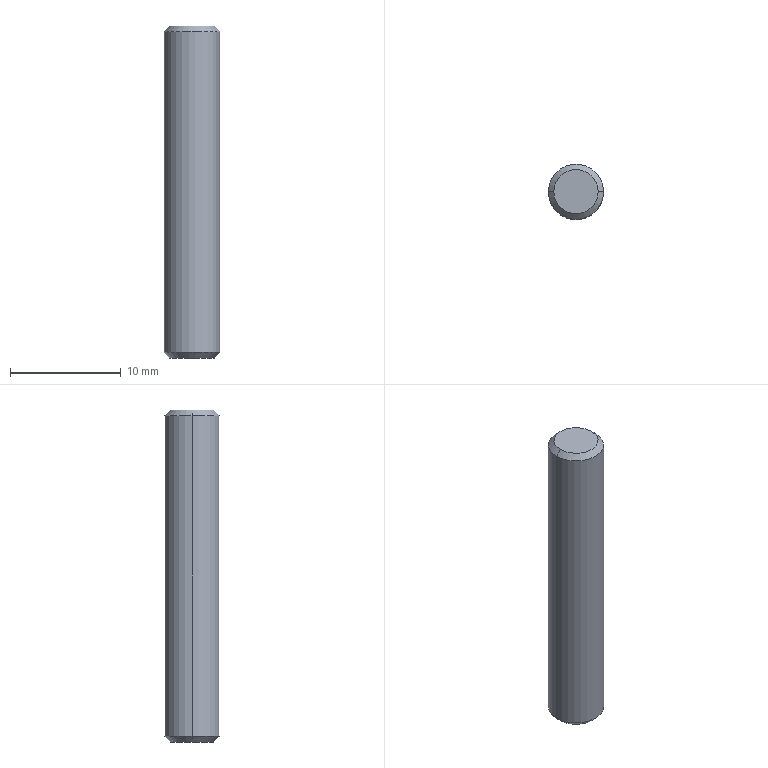Part | SolidWorks | features Chamfer 1, Extrusion 1 | 1 solid | 8 faces | box 5 x 5 x 30 mm | volume 585.383 mm3 | cone 4 | cylinder 2 | plane 2 | commonest cylinder face diameters 5 x2
STEP:
#1=CARTESIAN_POINT('',(-2.,0.,-15.));
#2=VERTEX_POINT('',#1);
#3=CARTESIAN_POINT('',(2.,0.,-15.));
#4=VERTEX_POINT('',#3);
#5=CARTESIAN_POINT('',(0.,0.,-15.));
#6=DIRECTION('',(0.,0.,-1.));
#7=DIRECTION('',(1.,0.,0.));
#8=AXIS2_PLACEMENT_3D('',#5,#6,#7);
#9=CIRCLE('',#8,2.);
#10=EDGE_CURVE('',#2,#4,#9,.T.);
#11=ORIENTED_EDGE('',*,*,#10,.F.);
#12=CARTESIAN_POINT('',(-2.5,0.,-14.5));
#13=VERTEX_POINT('',#12);
#14=CARTESIAN_POINT('',(-2.5,0.,-14.5));
#15=DIRECTION('',(-0.7071,0.,0.7071));
#16=VECTOR('',#15,1000.);
#17=LINE('',#14,#16);
#18=EDGE_CURVE('',#2,#13,#17,.T.);
#19=ORIENTED_EDGE('',*,*,#18,.T.);
#20=CARTESIAN_POINT('',(2.5,0.,-14.5));
#21=VERTEX_POINT('',#20);
#22=CARTESIAN_POINT('',(0.,0.,-14.5));
#23=DIRECTION('',(0.,0.,1.));
#24=DIRECTION('',(1.,0.,0.));
#25=AXIS2_PLACEMENT_3D('',#22,#23,#24);
#26=CIRCLE('',#25,2.5);
#27=EDGE_CURVE('',#21,#13,#26,.T.);
#28=ORIENTED_EDGE('',*,*,#27,.F.);
#29=CARTESIAN_POINT('',(2.5,0.,-14.5));
#30=DIRECTION('',(0.7071,0.,0.7071));
#31=VECTOR('',#30,1000.);
#32=LINE('',#29,#31);
#33=EDGE_CURVE('',#4,#21,#32,.T.);
#34=ORIENTED_EDGE('',*,*,#33,.F.);
#35=EDGE_LOOP('',(#11,#19,#28,#34));
#36=FACE_OUTER_BOUND('',#35,.T.);
#37=CARTESIAN_POINT('',(0.,0.,-14.5));
#38=DIRECTION('',(0.,0.,1.));
#39=DIRECTION('',(1.,0.,0.));
#40=AXIS2_PLACEMENT_3D('',#37,#38,#39);
#41=CONICAL_SURFACE('',#40,2.5,0.7854);
#42=ADVANCED_FACE('',(#36),#41,.T.);
#43=CARTESIAN_POINT('',(2.,0.,15.));
#44=VERTEX_POINT('',#43);
#45=CARTESIAN_POINT('',(-2.,0.,15.));
#46=VERTEX_POINT('',#45);
#47=CARTESIAN_POINT('',(0.,0.,15.));
#48=DIRECTION('',(0.,0.,1.));
#49=DIRECTION('',(1.,0.,0.));
#50=AXIS2_PLACEMENT_3D('',#47,#48,#49);
#51=CIRCLE('',#50,2.);
#52=EDGE_CURVE('',#44,#46,#51,.T.);
#53=ORIENTED_EDGE('',*,*,#52,.F.);
#54=CARTESIAN_POINT('',(2.5,0.,14.5));
#55=VERTEX_POINT('',#54);
#56=CARTESIAN_POINT('',(2.,0.,15.));
#57=DIRECTION('',(0.7071,0.,-0.7071));
#58=VECTOR('',#57,1000.);
#59=LINE('',#56,#58);
#60=EDGE_CURVE('',#44,#55,#59,.T.);
#61=ORIENTED_EDGE('',*,*,#60,.T.);
#62=CARTESIAN_POINT('',(-2.5,0.,14.5));
#63=VERTEX_POINT('',#62);
#64=CARTESIAN_POINT('',(0.,0.,14.5));
#65=DIRECTION('',(0.,0.,-1.));
#66=DIRECTION('',(1.,0.,0.));
#67=AXIS2_PLACEMENT_3D('',#64,#65,#66);
#68=CIRCLE('',#67,2.5);
#69=EDGE_CURVE('',#63,#55,#68,.T.);
#70=ORIENTED_EDGE('',*,*,#69,.F.);
#71=CARTESIAN_POINT('',(-2.,0.,15.));
#72=DIRECTION('',(-0.7071,0.,-0.7071));
#73=VECTOR('',#72,1000.);
#74=LINE('',#71,#73);
#75=EDGE_CURVE('',#46,#63,#74,.T.);
#76=ORIENTED_EDGE('',*,*,#75,.F.);
#77=EDGE_LOOP('',(#53,#61,#70,#76));
#78=FACE_OUTER_BOUND('',#77,.T.);
#79=CARTESIAN_POINT('',(0.,0.,15.));
#80=DIRECTION('',(0.,0.,-1.));
#81=DIRECTION('',(-1.,0.,0.));
#82=AXIS2_PLACEMENT_3D('',#79,#80,#81);
#83=CONICAL_SURFACE('',#82,2.,0.7854);
#84=ADVANCED_FACE('',(#78),#83,.T.);
#85=ORIENTED_EDGE('',*,*,#69,.T.);
#86=CARTESIAN_POINT('',(2.5,0.,15.));
#87=DIRECTION('',(0.,0.,-1.));
#88=VECTOR('',#87,1000.);
#89=LINE('',#86,#88);
#90=EDGE_CURVE('',#55,#21,#89,.T.);
#91=ORIENTED_EDGE('',*,*,#90,.T.);
#92=ORIENTED_EDGE('',*,*,#27,.T.);
#93=CARTESIAN_POINT('',(-2.5,0.,15.));
#94=DIRECTION('',(0.,0.,-1.));
#95=VECTOR('',#94,1000.);
#96=LINE('',#93,#95);
#97=EDGE_CURVE('',#63,#13,#96,.T.);
#98=ORIENTED_EDGE('',*,*,#97,.F.);
#99=EDGE_LOOP('',(#85,#91,#92,#98));
#100=FACE_OUTER_BOUND('',#99,.T.);
#101=CARTESIAN_POINT('',(0.,0.,15.));
#102=DIRECTION('',(0.,0.,-1.));
#103=DIRECTION('',(-1.,0.,0.));
#104=AXIS2_PLACEMENT_3D('',#101,#102,#103);
#105=CYLINDRICAL_SURFACE('',#104,2.5);
#106=ADVANCED_FACE('',(#100),#105,.T.);
#107=ORIENTED_EDGE('',*,*,#90,.F.);
#108=CARTESIAN_POINT('',(0.,0.,14.5));
#109=DIRECTION('',(0.,0.,-1.));
#110=DIRECTION('',(1.,0.,0.));
#111=AXIS2_PLACEMENT_3D('',#108,#109,#110);
#112=CIRCLE('',#111,2.5);
#113=EDGE_CURVE('',#55,#63,#112,.T.);
#114=ORIENTED_EDGE('',*,*,#113,.T.);
#115=ORIENTED_EDGE('',*,*,#97,.T.);
#116=CARTESIAN_POINT('',(0.,0.,-14.5));
#117=DIRECTION('',(0.,0.,1.));
#118=DIRECTION('',(1.,0.,0.));
#119=AXIS2_PLACEMENT_3D('',#116,#117,#118);
#120=CIRCLE('',#119,2.5);
#121=EDGE_CURVE('',#13,#21,#120,.T.);
#122=ORIENTED_EDGE('',*,*,#121,.T.);
#123=EDGE_LOOP('',(#107,#114,#115,#122));
#124=FACE_OUTER_BOUND('',#123,.T.);
#125=CARTESIAN_POINT('',(0.,0.,15.));
#126=DIRECTION('',(0.,0.,-1.));
#127=DIRECTION('',(-1.,0.,0.));
#128=AXIS2_PLACEMENT_3D('',#125,#126,#127);
#129=CYLINDRICAL_SURFACE('',#128,2.5);
#130=ADVANCED_FACE('',(#124),#129,.T.);
#131=CARTESIAN_POINT('',(0.,0.,15.));
#132=DIRECTION('',(0.,0.,1.));
#133=DIRECTION('',(1.,0.,0.));
#134=AXIS2_PLACEMENT_3D('',#131,#132,#133);
#135=CIRCLE('',#134,2.);
#136=EDGE_CURVE('',#46,#44,#135,.T.);
#137=ORIENTED_EDGE('',*,*,#136,.T.);
#138=ORIENTED_EDGE('',*,*,#52,.T.);
#139=EDGE_LOOP('',(#137,#138));
#140=FACE_OUTER_BOUND('',#139,.T.);
#141=CARTESIAN_POINT('',(0.,0.,15.));
#142=DIRECTION('',(0.,0.,1.));
#143=DIRECTION('',(1.,0.,0.));
#144=AXIS2_PLACEMENT_3D('',#141,#142,#143);
#145=PLANE('',#144);
#146=ADVANCED_FACE('',(#140),#145,.T.);
#147=CARTESIAN_POINT('',(0.,0.,-15.));
#148=DIRECTION('',(0.,0.,-1.));
#149=DIRECTION('',(1.,0.,0.));
#150=AXIS2_PLACEMENT_3D('',#147,#148,#149);
#151=CIRCLE('',#150,2.);
#152=EDGE_CURVE('',#4,#2,#151,.T.);
#153=ORIENTED_EDGE('',*,*,#152,.T.);
#154=ORIENTED_EDGE('',*,*,#10,.T.);
#155=EDGE_LOOP('',(#153,#154));
#156=FACE_OUTER_BOUND('',#155,.T.);
#157=CARTESIAN_POINT('',(0.,0.,-15.));
#158=DIRECTION('',(0.,0.,1.));
#159=DIRECTION('',(1.,0.,0.));
#160=AXIS2_PLACEMENT_3D('',#157,#158,#159);
#161=PLANE('',#160);
#162=ADVANCED_FACE('',(#156),#161,.F.);
#163=ORIENTED_EDGE('',*,*,#60,.F.);
#164=ORIENTED_EDGE('',*,*,#136,.F.);
#165=ORIENTED_EDGE('',*,*,#75,.T.);
#166=ORIENTED_EDGE('',*,*,#113,.F.);
#167=EDGE_LOOP('',(#163,#164,#165,#166));
#168=FACE_OUTER_BOUND('',#167,.T.);
#169=CARTESIAN_POINT('',(0.,0.,15.));
#170=DIRECTION('',(0.,0.,-1.));
#171=DIRECTION('',(-1.,0.,0.));
#172=AXIS2_PLACEMENT_3D('',#169,#170,#171);
#173=CONICAL_SURFACE('',#172,2.,0.7854);
#174=ADVANCED_FACE('',(#168),#173,.T.);
#175=ORIENTED_EDGE('',*,*,#18,.F.);
#176=ORIENTED_EDGE('',*,*,#152,.F.);
#177=ORIENTED_EDGE('',*,*,#33,.T.);
#178=ORIENTED_EDGE('',*,*,#121,.F.);
#179=EDGE_LOOP('',(#175,#176,#177,#178));
#180=FACE_OUTER_BOUND('',#179,.T.);
#181=CARTESIAN_POINT('',(0.,0.,-14.5));
#182=DIRECTION('',(0.,0.,1.));
#183=DIRECTION('',(1.,0.,0.));
#184=AXIS2_PLACEMENT_3D('',#181,#182,#183);
#185=CONICAL_SURFACE('',#184,2.5,0.7854);
#186=ADVANCED_FACE('',(#180),#185,.T.);
#187=CLOSED_SHELL('',(#42,#84,#106,#130,#146,#162,#174,#186));
#188=MANIFOLD_SOLID_BREP('',#187);
#189=CARTESIAN_POINT('',(0.,0.,0.));
#190=DIRECTION('',(0.,0.,1.));
#191=DIRECTION('',(1.,0.,0.));
#192=AXIS2_PLACEMENT_3D('',#189,#190,#191);
#193=(LENGTH_UNIT()NAMED_UNIT(*)SI_UNIT(.MILLI.,.METRE.));
#194=UNCERTAINTY_MEASURE_WITH_UNIT(LENGTH_MEASURE(0.00001),#193,'','');
#195=(NAMED_UNIT(*)PLANE_ANGLE_UNIT()SI_UNIT($,.RADIAN.));
#196=(NAMED_UNIT(*)SI_UNIT($,.STERADIAN.)SOLID_ANGLE_UNIT());
#197=(GEOMETRIC_REPRESENTATION_CONTEXT(3)GLOBAL_UNCERTAINTY_ASSIGNED_CONTEXT((#194))GLOBAL_UNIT_ASSIGNED_CONTEXT((#193,#195,#196))REPRESENTATION_CONTEXT('',''));
#198=ADVANCED_BREP_SHAPE_REPRESENTATION('',(#188,#192),#197);